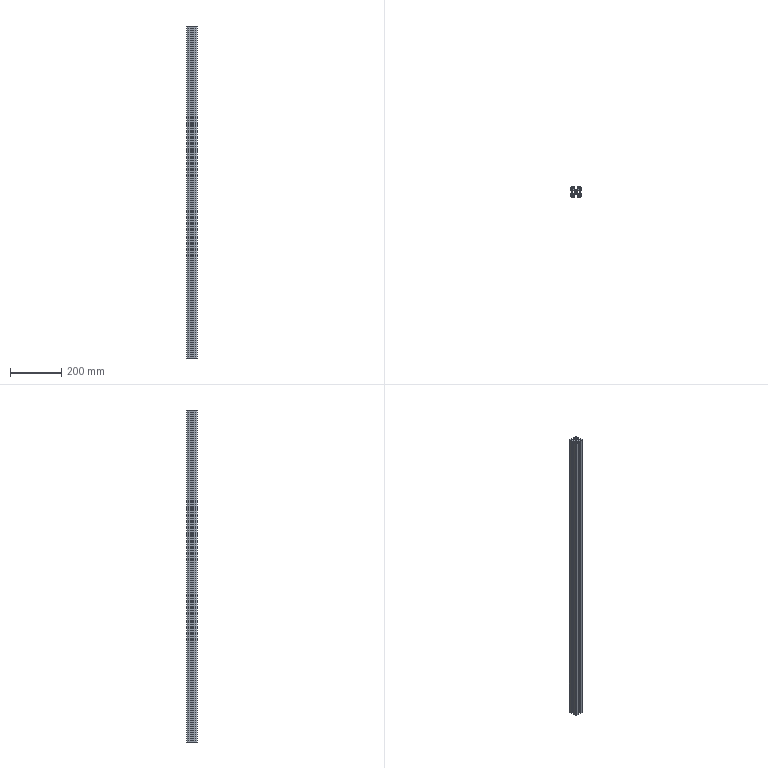Part | STEP file | HM-8-4040D-L1300 | 1 solid | 176 faces | box 40 x 40 x 1300 mm | volume 890054 mm3 | plane 90 | cylinder 86 | commonest cylinder face diameters 1 x40 0.4 x24 4 x8 6 x8 9 x4 6.8 x2